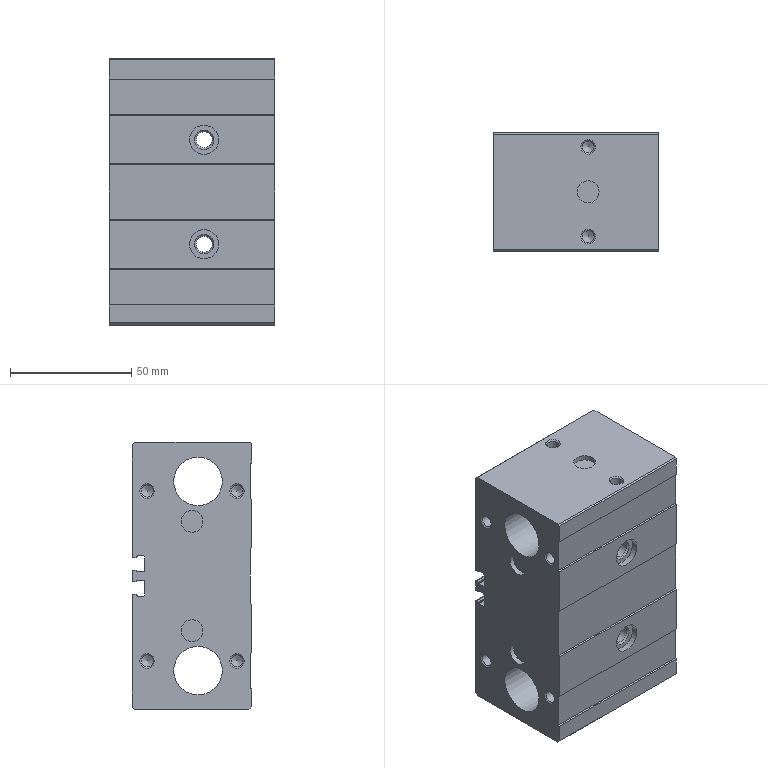Part | NX | features BREP 1 | 1 solid | 114 faces | box 68 x 49.05 x 110 mm | volume 271121 mm3 | plane 54 | cylinder 42 | cone 18 | commonest cylinder face diameters 0.4 x8 0.8 x8 4.917 x6 8.566 x4 9 x3 12 x3